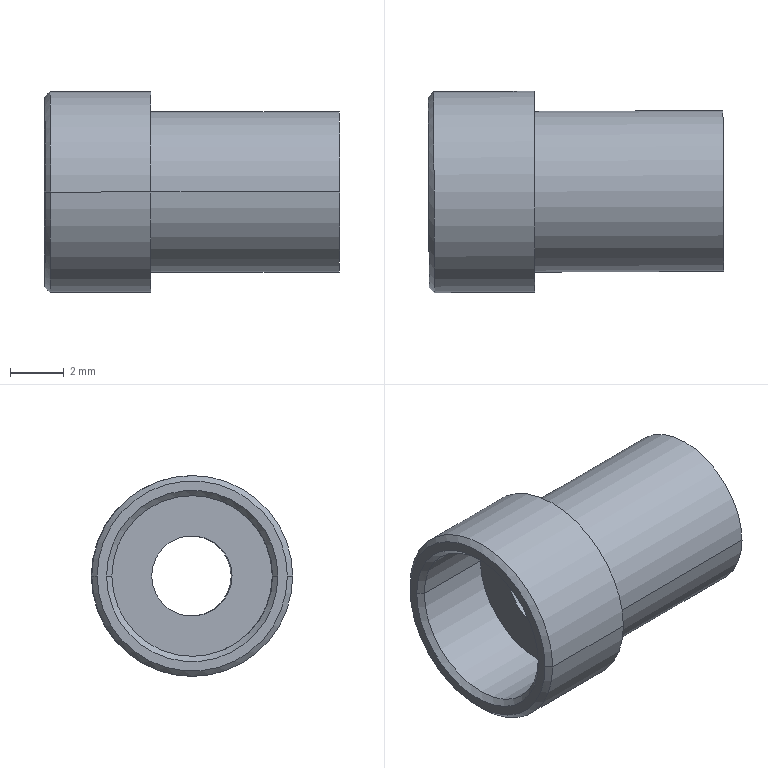Part | SolidWorks | features BaseBody 1 | 1 solid | 16 faces | box 11.028 x 7.516 x 7.5 mm | volume 227.909 mm3 | cylinder 8 | cone 4 | plane 4 | commonest cylinder face diameters 6 x4 3 x2 7.5 x2
STEP:
#1=CARTESIAN_POINT('',(582.359,67.257,169.293));
#2=VERTEX_POINT('',#1);
#3=CARTESIAN_POINT('',(582.385,61.257,169.293));
#4=VERTEX_POINT('',#3);
#5=CARTESIAN_POINT('',(582.372,64.257,169.293));
#6=DIRECTION('',(1.,0.004352,0.000000013));
#7=DIRECTION('',(-0.004352,1.,0.));
#8=AXIS2_PLACEMENT_3D('',#5,#6,#7);
#9=CIRCLE('',#8,3.);
#10=EDGE_CURVE('',#2,#4,#9,.T.);
#11=ORIENTED_EDGE('',*,*,#10,.T.);
#12=CARTESIAN_POINT('',(589.435,61.288,169.293));
#13=VERTEX_POINT('',#12);
#14=CARTESIAN_POINT('',(582.385,61.257,169.293));
#15=DIRECTION('',(1.,0.004352,0.000000013));
#16=VECTOR('',#15,1000.);
#17=LINE('',#14,#16);
#18=EDGE_CURVE('',#4,#13,#17,.T.);
#19=ORIENTED_EDGE('',*,*,#18,.T.);
#20=CARTESIAN_POINT('',(589.409,67.288,169.293));
#21=VERTEX_POINT('',#20);
#22=CARTESIAN_POINT('',(589.422,64.288,169.293));
#23=DIRECTION('',(-1.,-0.004352,-0.000000013));
#24=DIRECTION('',(-0.004352,1.,0.));
#25=AXIS2_PLACEMENT_3D('',#22,#23,#24);
#26=CIRCLE('',#25,3.);
#27=EDGE_CURVE('',#13,#21,#26,.T.);
#28=ORIENTED_EDGE('',*,*,#27,.T.);
#29=CARTESIAN_POINT('',(582.359,67.257,169.293));
#30=DIRECTION('',(1.,0.004352,0.000000013));
#31=VECTOR('',#30,1000.);
#32=LINE('',#29,#31);
#33=EDGE_CURVE('',#2,#21,#32,.T.);
#34=ORIENTED_EDGE('',*,*,#33,.F.);
#35=EDGE_LOOP('',(#11,#19,#28,#34));
#36=FACE_OUTER_BOUND('',#35,.T.);
#37=CARTESIAN_POINT('',(582.372,64.257,169.293));
#38=DIRECTION('',(1.,0.004352,0.000000013));
#39=DIRECTION('',(-0.004352,1.,0.));
#40=AXIS2_PLACEMENT_3D('',#37,#38,#39);
#41=CYLINDRICAL_SURFACE('',#40,3.);
#42=ADVANCED_FACE('',(#36),#41,.T.);
#43=CARTESIAN_POINT('',(581.604,62.754,169.293));
#44=VERTEX_POINT('',#43);
#45=CARTESIAN_POINT('',(581.591,65.754,169.293));
#46=VERTEX_POINT('',#45);
#47=CARTESIAN_POINT('',(581.597,64.254,169.293));
#48=DIRECTION('',(1.,0.004352,0.000000013));
#49=DIRECTION('',(-0.004352,1.,0.));
#50=AXIS2_PLACEMENT_3D('',#47,#48,#49);
#51=CIRCLE('',#50,1.5);
#52=EDGE_CURVE('',#44,#46,#51,.T.);
#53=ORIENTED_EDGE('',*,*,#52,.F.);
#54=CARTESIAN_POINT('',(589.429,62.788,169.293));
#55=VERTEX_POINT('',#54);
#56=CARTESIAN_POINT('',(586.016,62.773,169.293));
#57=DIRECTION('',(1.,0.004352,0.000000013));
#58=VECTOR('',#57,1000.);
#59=LINE('',#56,#58);
#60=EDGE_CURVE('',#44,#55,#59,.T.);
#61=ORIENTED_EDGE('',*,*,#60,.T.);
#62=CARTESIAN_POINT('',(589.416,65.788,169.293));
#63=VERTEX_POINT('',#62);
#64=CARTESIAN_POINT('',(589.422,64.288,169.293));
#65=DIRECTION('',(-1.,-0.004352,-0.000000013));
#66=DIRECTION('',(-0.004352,1.,0.));
#67=AXIS2_PLACEMENT_3D('',#64,#65,#66);
#68=CIRCLE('',#67,1.5);
#69=EDGE_CURVE('',#63,#55,#68,.T.);
#70=ORIENTED_EDGE('',*,*,#69,.F.);
#71=CARTESIAN_POINT('',(586.003,65.773,169.293));
#72=DIRECTION('',(1.,0.004352,0.000000013));
#73=VECTOR('',#72,1000.);
#74=LINE('',#71,#73);
#75=EDGE_CURVE('',#46,#63,#74,.T.);
#76=ORIENTED_EDGE('',*,*,#75,.F.);
#77=EDGE_LOOP('',(#53,#61,#70,#76));
#78=FACE_OUTER_BOUND('',#77,.T.);
#79=CARTESIAN_POINT('',(586.01,64.273,169.293));
#80=DIRECTION('',(1.,0.004352,0.000000013));
#81=DIRECTION('',(-0.004352,1.,0.));
#82=AXIS2_PLACEMENT_3D('',#79,#80,#81);
#83=CYLINDRICAL_SURFACE('',#82,1.5);
#84=ADVANCED_FACE('',(#78),#83,.F.);
#85=CARTESIAN_POINT('',(582.389,60.507,169.293));
#86=VERTEX_POINT('',#85);
#87=CARTESIAN_POINT('',(582.356,68.007,169.293));
#88=VERTEX_POINT('',#87);
#89=CARTESIAN_POINT('',(582.372,64.257,169.293));
#90=DIRECTION('',(-1.,-0.004352,-0.000000013));
#91=DIRECTION('',(0.004352,-1.,0.));
#92=AXIS2_PLACEMENT_3D('',#89,#90,#91);
#93=CIRCLE('',#92,3.75);
#94=EDGE_CURVE('',#86,#88,#93,.T.);
#95=ORIENTED_EDGE('',*,*,#94,.T.);
#96=CARTESIAN_POINT('',(578.606,67.991,169.293));
#97=VERTEX_POINT('',#96);
#98=CARTESIAN_POINT('',(582.356,68.007,169.293));
#99=DIRECTION('',(-1.,-0.004352,-0.000000013));
#100=VECTOR('',#99,1000.);
#101=LINE('',#98,#100);
#102=EDGE_CURVE('',#88,#97,#101,.T.);
#103=ORIENTED_EDGE('',*,*,#102,.T.);
#104=CARTESIAN_POINT('',(578.639,60.491,169.293));
#105=VERTEX_POINT('',#104);
#106=CARTESIAN_POINT('',(578.622,64.241,169.293));
#107=DIRECTION('',(1.,0.004352,0.000000013));
#108=DIRECTION('',(0.004352,-1.,0.));
#109=AXIS2_PLACEMENT_3D('',#106,#107,#108);
#110=CIRCLE('',#109,3.75);
#111=EDGE_CURVE('',#97,#105,#110,.T.);
#112=ORIENTED_EDGE('',*,*,#111,.T.);
#113=CARTESIAN_POINT('',(582.389,60.507,169.293));
#114=DIRECTION('',(-1.,-0.004352,-0.000000013));
#115=VECTOR('',#114,1000.);
#116=LINE('',#113,#115);
#117=EDGE_CURVE('',#86,#105,#116,.T.);
#118=ORIENTED_EDGE('',*,*,#117,.F.);
#119=EDGE_LOOP('',(#95,#103,#112,#118));
#120=FACE_OUTER_BOUND('',#119,.T.);
#121=CARTESIAN_POINT('',(582.372,64.257,169.293));
#122=DIRECTION('',(-1.,-0.004352,-0.000000013));
#123=DIRECTION('',(0.004352,-1.,0.));
#124=AXIS2_PLACEMENT_3D('',#121,#122,#123);
#125=CYLINDRICAL_SURFACE('',#124,3.75);
#126=ADVANCED_FACE('',(#120),#125,.T.);
#127=CARTESIAN_POINT('',(578.407,67.79,169.293));
#128=VERTEX_POINT('',#127);
#129=CARTESIAN_POINT('',(578.438,60.69,169.293));
#130=VERTEX_POINT('',#129);
#131=CARTESIAN_POINT('',(578.422,64.24,169.293));
#132=DIRECTION('',(1.,0.004352,0.000000013));
#133=DIRECTION('',(-0.004352,1.,0.));
#134=AXIS2_PLACEMENT_3D('',#131,#132,#133);
#135=CIRCLE('',#134,3.55);
#136=EDGE_CURVE('',#128,#130,#135,.T.);
#137=ORIENTED_EDGE('',*,*,#136,.T.);
#138=CARTESIAN_POINT('',(578.639,60.491,169.293));
#139=DIRECTION('',(0.7102,-0.704,0.000000009));
#140=VECTOR('',#139,1000.);
#141=LINE('',#138,#140);
#142=EDGE_CURVE('',#130,#105,#141,.T.);
#143=ORIENTED_EDGE('',*,*,#142,.T.);
#144=ORIENTED_EDGE('',*,*,#111,.F.);
#145=CARTESIAN_POINT('',(578.606,67.991,169.293));
#146=DIRECTION('',(0.704,0.7102,0.000000009));
#147=VECTOR('',#146,1000.);
#148=LINE('',#145,#147);
#149=EDGE_CURVE('',#128,#97,#148,.T.);
#150=ORIENTED_EDGE('',*,*,#149,.F.);
#151=EDGE_LOOP('',(#137,#143,#144,#150));
#152=FACE_OUTER_BOUND('',#151,.T.);
#153=CARTESIAN_POINT('',(578.622,64.241,169.293));
#154=DIRECTION('',(1.,0.004352,0.000000013));
#155=DIRECTION('',(-0.004352,1.,0.));
#156=AXIS2_PLACEMENT_3D('',#153,#154,#155);
#157=CONICAL_SURFACE('',#156,3.75,0.7854);
#158=ADVANCED_FACE('',(#152),#157,.T.);
#159=CARTESIAN_POINT('',(578.635,61.241,169.293));
#160=VERTEX_POINT('',#159);
#161=CARTESIAN_POINT('',(578.609,67.241,169.293));
#162=VERTEX_POINT('',#161);
#163=CARTESIAN_POINT('',(578.622,64.241,169.293));
#164=DIRECTION('',(1.,0.004352,0.000000013));
#165=DIRECTION('',(-0.004352,1.,0.));
#166=AXIS2_PLACEMENT_3D('',#163,#164,#165);
#167=CIRCLE('',#166,3.);
#168=EDGE_CURVE('',#160,#162,#167,.T.);
#169=ORIENTED_EDGE('',*,*,#168,.F.);
#170=CARTESIAN_POINT('',(581.61,61.254,169.293));
#171=VERTEX_POINT('',#170);
#172=CARTESIAN_POINT('',(580.023,61.247,169.293));
#173=DIRECTION('',(1.,0.004352,0.000000013));
#174=VECTOR('',#173,1000.);
#175=LINE('',#172,#174);
#176=EDGE_CURVE('',#160,#171,#175,.T.);
#177=ORIENTED_EDGE('',*,*,#176,.T.);
#178=CARTESIAN_POINT('',(581.584,67.254,169.293));
#179=VERTEX_POINT('',#178);
#180=CARTESIAN_POINT('',(581.597,64.254,169.293));
#181=DIRECTION('',(1.,0.004352,0.000000013));
#182=DIRECTION('',(-0.004352,1.,0.));
#183=AXIS2_PLACEMENT_3D('',#180,#181,#182);
#184=CIRCLE('',#183,3.);
#185=EDGE_CURVE('',#171,#179,#184,.T.);
#186=ORIENTED_EDGE('',*,*,#185,.T.);
#187=CARTESIAN_POINT('',(579.997,67.247,169.293));
#188=DIRECTION('',(1.,0.004352,0.000000013));
#189=VECTOR('',#188,1000.);
#190=LINE('',#187,#189);
#191=EDGE_CURVE('',#162,#179,#190,.T.);
#192=ORIENTED_EDGE('',*,*,#191,.F.);
#193=EDGE_LOOP('',(#169,#177,#186,#192));
#194=FACE_OUTER_BOUND('',#193,.T.);
#195=CARTESIAN_POINT('',(580.01,64.247,169.293));
#196=DIRECTION('',(1.,0.004352,0.000000013));
#197=DIRECTION('',(-0.004352,1.,0.));
#198=AXIS2_PLACEMENT_3D('',#195,#196,#197);
#199=CYLINDRICAL_SURFACE('',#198,3.);
#200=ADVANCED_FACE('',(#194),#199,.F.);
#201=ORIENTED_EDGE('',*,*,#168,.T.);
#202=CARTESIAN_POINT('',(578.408,67.44,169.293));
#203=VERTEX_POINT('',#202);
#204=CARTESIAN_POINT('',(578.408,67.44,169.293));
#205=DIRECTION('',(-0.7102,0.704,-0.000000009));
#206=VECTOR('',#205,1000.);
#207=LINE('',#204,#206);
#208=EDGE_CURVE('',#162,#203,#207,.T.);
#209=ORIENTED_EDGE('',*,*,#208,.T.);
#210=CARTESIAN_POINT('',(578.436,61.04,169.293));
#211=VERTEX_POINT('',#210);
#212=CARTESIAN_POINT('',(578.422,64.24,169.293));
#213=DIRECTION('',(1.,0.004352,0.000000013));
#214=DIRECTION('',(0.004352,-1.,0.));
#215=AXIS2_PLACEMENT_3D('',#212,#213,#214);
#216=CIRCLE('',#215,3.2);
#217=EDGE_CURVE('',#211,#203,#216,.T.);
#218=ORIENTED_EDGE('',*,*,#217,.F.);
#219=CARTESIAN_POINT('',(578.436,61.04,169.293));
#220=DIRECTION('',(-0.704,-0.7102,-0.000000009));
#221=VECTOR('',#220,1000.);
#222=LINE('',#219,#221);
#223=EDGE_CURVE('',#160,#211,#222,.T.);
#224=ORIENTED_EDGE('',*,*,#223,.F.);
#225=EDGE_LOOP('',(#201,#209,#218,#224));
#226=FACE_OUTER_BOUND('',#225,.T.);
#227=CARTESIAN_POINT('',(578.422,64.24,169.293));
#228=DIRECTION('',(-1.,-0.004352,-0.000000013));
#229=DIRECTION('',(0.004352,-1.,0.));
#230=AXIS2_PLACEMENT_3D('',#227,#228,#229);
#231=CONICAL_SURFACE('',#230,3.2,0.7854);
#232=ADVANCED_FACE('',(#226),#231,.F.);
#233=ORIENTED_EDGE('',*,*,#18,.F.);
#234=CARTESIAN_POINT('',(582.372,64.257,169.293));
#235=DIRECTION('',(1.,0.004352,0.000000013));
#236=DIRECTION('',(-0.004352,1.,0.));
#237=AXIS2_PLACEMENT_3D('',#234,#235,#236);
#238=CIRCLE('',#237,3.);
#239=EDGE_CURVE('',#4,#2,#238,.T.);
#240=ORIENTED_EDGE('',*,*,#239,.T.);
#241=ORIENTED_EDGE('',*,*,#33,.T.);
#242=CARTESIAN_POINT('',(589.422,64.288,169.293));
#243=DIRECTION('',(-1.,-0.004352,-0.000000013));
#244=DIRECTION('',(-0.004352,1.,0.));
#245=AXIS2_PLACEMENT_3D('',#242,#243,#244);
#246=CIRCLE('',#245,3.);
#247=EDGE_CURVE('',#21,#13,#246,.T.);
#248=ORIENTED_EDGE('',*,*,#247,.T.);
#249=EDGE_LOOP('',(#233,#240,#241,#248));
#250=FACE_OUTER_BOUND('',#249,.T.);
#251=CARTESIAN_POINT('',(582.372,64.257,169.293));
#252=DIRECTION('',(1.,0.004352,0.000000013));
#253=DIRECTION('',(-0.004352,1.,0.));
#254=AXIS2_PLACEMENT_3D('',#251,#252,#253);
#255=CYLINDRICAL_SURFACE('',#254,3.);
#256=ADVANCED_FACE('',(#250),#255,.T.);
#257=ORIENTED_EDGE('',*,*,#247,.F.);
#258=ORIENTED_EDGE('',*,*,#27,.F.);
#259=EDGE_LOOP('',(#257,#258));
#260=FACE_OUTER_BOUND('',#259,.T.);
#261=ORIENTED_EDGE('',*,*,#69,.T.);
#262=CARTESIAN_POINT('',(589.422,64.288,169.293));
#263=DIRECTION('',(-1.,-0.004352,-0.000000013));
#264=DIRECTION('',(-0.004352,1.,0.));
#265=AXIS2_PLACEMENT_3D('',#262,#263,#264);
#266=CIRCLE('',#265,1.5);
#267=EDGE_CURVE('',#55,#63,#266,.T.);
#268=ORIENTED_EDGE('',*,*,#267,.T.);
#269=EDGE_LOOP('',(#261,#268));
#270=FACE_BOUND('',#269,.T.);
#271=CARTESIAN_POINT('',(589.422,64.288,169.293));
#272=DIRECTION('',(1.,0.004352,0.000000013));
#273=DIRECTION('',(-0.004352,1.,0.));
#274=AXIS2_PLACEMENT_3D('',#271,#272,#273);
#275=PLANE('',#274);
#276=ADVANCED_FACE('',(#260,#270),#275,.T.);
#277=ORIENTED_EDGE('',*,*,#10,.F.);
#278=ORIENTED_EDGE('',*,*,#239,.F.);
#279=EDGE_LOOP('',(#277,#278));
#280=FACE_BOUND('',#279,.T.);
#281=ORIENTED_EDGE('',*,*,#94,.F.);
#282=CARTESIAN_POINT('',(582.372,64.257,169.293));
#283=DIRECTION('',(-1.,-0.004352,-0.000000013));
#284=DIRECTION('',(0.004352,-1.,0.));
#285=AXIS2_PLACEMENT_3D('',#282,#283,#284);
#286=CIRCLE('',#285,3.75);
#287=EDGE_CURVE('',#88,#86,#286,.T.);
#288=ORIENTED_EDGE('',*,*,#287,.F.);
#289=EDGE_LOOP('',(#281,#288));
#290=FACE_OUTER_BOUND('',#289,.T.);
#291=CARTESIAN_POINT('',(582.372,64.257,169.293));
#292=DIRECTION('',(-1.,-0.004352,-0.000000013));
#293=DIRECTION('',(0.004352,-1.,0.));
#294=AXIS2_PLACEMENT_3D('',#291,#292,#293);
#295=PLANE('',#294);
#296=ADVANCED_FACE('',(#280,#290),#295,.F.);
#297=ORIENTED_EDGE('',*,*,#60,.F.);
#298=CARTESIAN_POINT('',(581.597,64.254,169.293));
#299=DIRECTION('',(1.,0.004352,0.000000013));
#300=DIRECTION('',(-0.004352,1.,0.));
#301=AXIS2_PLACEMENT_3D('',#298,#299,#300);
#302=CIRCLE('',#301,1.5);
#303=EDGE_CURVE('',#46,#44,#302,.T.);
#304=ORIENTED_EDGE('',*,*,#303,.F.);
#305=ORIENTED_EDGE('',*,*,#75,.T.);
#306=ORIENTED_EDGE('',*,*,#267,.F.);
#307=EDGE_LOOP('',(#297,#304,#305,#306));
#308=FACE_OUTER_BOUND('',#307,.T.);
#309=CARTESIAN_POINT('',(586.01,64.273,169.293));
#310=DIRECTION('',(1.,0.004352,0.000000013));
#311=DIRECTION('',(-0.004352,1.,0.));
#312=AXIS2_PLACEMENT_3D('',#309,#310,#311);
#313=CYLINDRICAL_SURFACE('',#312,1.5);
#314=ADVANCED_FACE('',(#308),#313,.F.);
#315=ORIENTED_EDGE('',*,*,#102,.F.);
#316=ORIENTED_EDGE('',*,*,#287,.T.);
#317=ORIENTED_EDGE('',*,*,#117,.T.);
#318=CARTESIAN_POINT('',(578.622,64.241,169.293));
#319=DIRECTION('',(1.,0.004352,0.000000013));
#320=DIRECTION('',(0.004352,-1.,0.));
#321=AXIS2_PLACEMENT_3D('',#318,#319,#320);
#322=CIRCLE('',#321,3.75);
#323=EDGE_CURVE('',#105,#97,#322,.T.);
#324=ORIENTED_EDGE('',*,*,#323,.T.);
#325=EDGE_LOOP('',(#315,#316,#317,#324));
#326=FACE_OUTER_BOUND('',#325,.T.);
#327=CARTESIAN_POINT('',(582.372,64.257,169.293));
#328=DIRECTION('',(-1.,-0.004352,-0.000000013));
#329=DIRECTION('',(0.004352,-1.,0.));
#330=AXIS2_PLACEMENT_3D('',#327,#328,#329);
#331=CYLINDRICAL_SURFACE('',#330,3.75);
#332=ADVANCED_FACE('',(#326),#331,.T.);
#333=CARTESIAN_POINT('',(581.597,64.254,169.293));
#334=DIRECTION('',(1.,0.004352,0.000000013));
#335=DIRECTION('',(-0.004352,1.,0.));
#336=AXIS2_PLACEMENT_3D('',#333,#334,#335);
#337=CIRCLE('',#336,3.);
#338=EDGE_CURVE('',#179,#171,#337,.T.);
#339=ORIENTED_EDGE('',*,*,#338,.F.);
#340=ORIENTED_EDGE('',*,*,#185,.F.);
#341=EDGE_LOOP('',(#339,#340));
#342=FACE_OUTER_BOUND('',#341,.T.);
#343=ORIENTED_EDGE('',*,*,#303,.T.);
#344=ORIENTED_EDGE('',*,*,#52,.T.);
#345=EDGE_LOOP('',(#343,#344));
#346=FACE_BOUND('',#345,.T.);
#347=CARTESIAN_POINT('',(581.607,62.029,168.961));
#348=DIRECTION('',(1.,0.004352,0.000000013));
#349=DIRECTION('',(-0.004352,1.,0.));
#350=AXIS2_PLACEMENT_3D('',#347,#348,#349);
#351=PLANE('',#350);
#352=ADVANCED_FACE('',(#342,#346),#351,.F.);
#353=ORIENTED_EDGE('',*,*,#142,.F.);
#354=CARTESIAN_POINT('',(578.422,64.24,169.293));
#355=DIRECTION('',(1.,0.004352,0.000000013));
#356=DIRECTION('',(-0.004352,1.,0.));
#357=AXIS2_PLACEMENT_3D('',#354,#355,#356);
#358=CIRCLE('',#357,3.55);
#359=EDGE_CURVE('',#130,#128,#358,.T.);
#360=ORIENTED_EDGE('',*,*,#359,.T.);
#361=ORIENTED_EDGE('',*,*,#149,.T.);
#362=ORIENTED_EDGE('',*,*,#323,.F.);
#363=EDGE_LOOP('',(#353,#360,#361,#362));
#364=FACE_OUTER_BOUND('',#363,.T.);
#365=CARTESIAN_POINT('',(578.622,64.241,169.293));
#366=DIRECTION('',(1.,0.004352,0.000000013));
#367=DIRECTION('',(-0.004352,1.,0.));
#368=AXIS2_PLACEMENT_3D('',#365,#366,#367);
#369=CONICAL_SURFACE('',#368,3.75,0.7854);
#370=ADVANCED_FACE('',(#364),#369,.T.);
#371=ORIENTED_EDGE('',*,*,#176,.F.);
#372=CARTESIAN_POINT('',(578.622,64.241,169.293));
#373=DIRECTION('',(1.,0.004352,0.000000013));
#374=DIRECTION('',(-0.004352,1.,0.));
#375=AXIS2_PLACEMENT_3D('',#372,#373,#374);
#376=CIRCLE('',#375,3.);
#377=EDGE_CURVE('',#162,#160,#376,.T.);
#378=ORIENTED_EDGE('',*,*,#377,.F.);
#379=ORIENTED_EDGE('',*,*,#191,.T.);
#380=ORIENTED_EDGE('',*,*,#338,.T.);
#381=EDGE_LOOP('',(#371,#378,#379,#380));
#382=FACE_OUTER_BOUND('',#381,.T.);
#383=CARTESIAN_POINT('',(580.01,64.247,169.293));
#384=DIRECTION('',(1.,0.004352,0.000000013));
#385=DIRECTION('',(-0.004352,1.,0.));
#386=AXIS2_PLACEMENT_3D('',#383,#384,#385);
#387=CYLINDRICAL_SURFACE('',#386,3.);
#388=ADVANCED_FACE('',(#382),#387,.F.);
#389=ORIENTED_EDGE('',*,*,#217,.T.);
#390=CARTESIAN_POINT('',(578.422,64.24,169.293));
#391=DIRECTION('',(1.,0.004352,0.000000013));
#392=DIRECTION('',(0.004352,-1.,0.));
#393=AXIS2_PLACEMENT_3D('',#390,#391,#392);
#394=CIRCLE('',#393,3.2);
#395=EDGE_CURVE('',#203,#211,#394,.T.);
#396=ORIENTED_EDGE('',*,*,#395,.T.);
#397=EDGE_LOOP('',(#389,#396));
#398=FACE_BOUND('',#397,.T.);
#399=ORIENTED_EDGE('',*,*,#136,.F.);
#400=ORIENTED_EDGE('',*,*,#359,.F.);
#401=EDGE_LOOP('',(#399,#400));
#402=FACE_OUTER_BOUND('',#401,.T.);
#403=CARTESIAN_POINT('',(578.422,64.24,169.293));
#404=DIRECTION('',(-1.,-0.004352,-0.000000013));
#405=DIRECTION('',(0.004352,-1.,0.));
#406=AXIS2_PLACEMENT_3D('',#403,#404,#405);
#407=PLANE('',#406);
#408=ADVANCED_FACE('',(#398,#402),#407,.T.);
#409=ORIENTED_EDGE('',*,*,#208,.F.);
#410=ORIENTED_EDGE('',*,*,#377,.T.);
#411=ORIENTED_EDGE('',*,*,#223,.T.);
#412=ORIENTED_EDGE('',*,*,#395,.F.);
#413=EDGE_LOOP('',(#409,#410,#411,#412));
#414=FACE_OUTER_BOUND('',#413,.T.);
#415=CARTESIAN_POINT('',(578.422,64.24,169.293));
#416=DIRECTION('',(-1.,-0.004352,-0.000000013));
#417=DIRECTION('',(0.004352,-1.,0.));
#418=AXIS2_PLACEMENT_3D('',#415,#416,#417);
#419=CONICAL_SURFACE('',#418,3.2,0.7854);
#420=ADVANCED_FACE('',(#414),#419,.F.);
#421=CLOSED_SHELL('',(#42,#84,#126,#158,#200,#232,#256,#276,#296,#314,#332,#352,#370,#388,#408,#420));
#422=MANIFOLD_SOLID_BREP('',#421);
#423=CARTESIAN_POINT('',(0.,0.,0.));
#424=DIRECTION('',(0.,0.,1.));
#425=DIRECTION('',(1.,0.,0.));
#426=AXIS2_PLACEMENT_3D('',#423,#424,#425);
#427=(LENGTH_UNIT()NAMED_UNIT(*)SI_UNIT(.MILLI.,.METRE.));
#428=UNCERTAINTY_MEASURE_WITH_UNIT(LENGTH_MEASURE(0.00001),#427,'','');
#429=(NAMED_UNIT(*)PLANE_ANGLE_UNIT()SI_UNIT($,.RADIAN.));
#430=(NAMED_UNIT(*)SI_UNIT($,.STERADIAN.)SOLID_ANGLE_UNIT());
#431=(GEOMETRIC_REPRESENTATION_CONTEXT(3)GLOBAL_UNCERTAINTY_ASSIGNED_CONTEXT((#428))GLOBAL_UNIT_ASSIGNED_CONTEXT((#427,#429,#430))REPRESENTATION_CONTEXT('',''));
#432=ADVANCED_BREP_SHAPE_REPRESENTATION('',(#422,#426),#431);